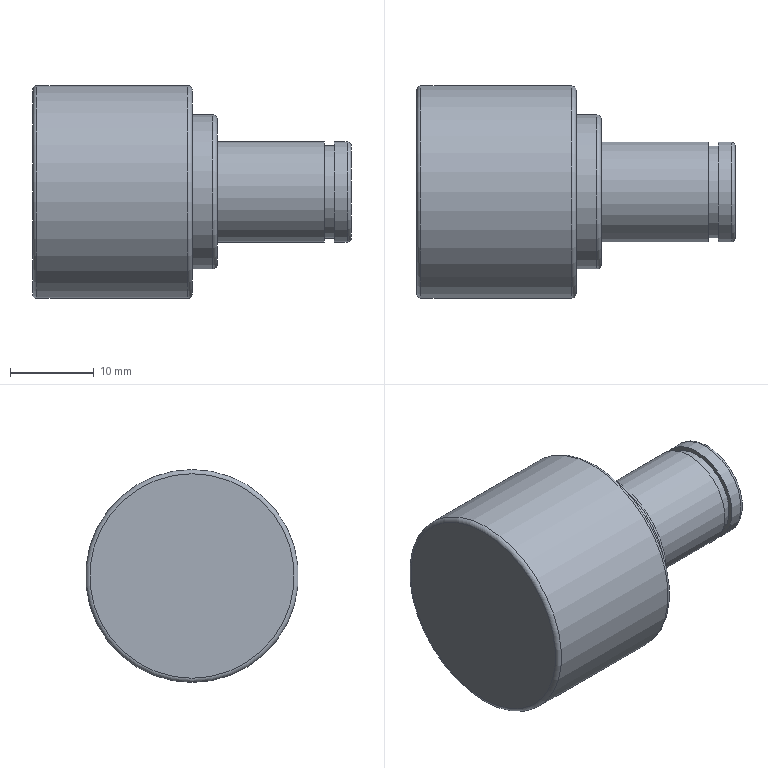Part | STEP file | 6100506 | 1 solid | 15 faces | box 38 x 25.4 x 25.4 mm | volume 12200 mm3 | plane 6 | cylinder 5 | torus 4 | commonest cylinder face diameters 12 x2 11 x1 18.4 x1 25.4 x1
STEP:
#1=CARTESIAN_POINT('',(0.,0.,0.));
#2=DIRECTION('',(0.,0.,1.));
#3=DIRECTION('',(1.,0.,0.));
#4=AXIS2_PLACEMENT_3D('',#1,#2,#3);
#5=CARTESIAN_POINT('',(0.,0.,12.2));
#6=VERTEX_POINT('',#5);
#7=CARTESIAN_POINT('',(0.,0.,0.));
#8=DIRECTION('',(-1.,0.,0.));
#9=DIRECTION('',(0.,0.,1.));
#10=AXIS2_PLACEMENT_3D('',#7,#8,#9);
#11=CIRCLE('',#10,12.2);
#12=CARTESIAN_POINT('',(0.,0.,0.));
#13=DIRECTION('',(1.,0.,0.));
#14=DIRECTION('',(0.,0.,-1.));
#15=AXIS2_PLACEMENT_3D('',#12,#13,#14);
#16=PLANE('',#15);
#17=CARTESIAN_POINT('',(-12.2,0.));
#18=CARTESIAN_POINT('',(-12.2,21.131));
#19=CARTESIAN_POINT('',(6.1,10.566));
#20=CARTESIAN_POINT('',(24.4,0.));
#21=CARTESIAN_POINT('',(6.1,-10.566));
#22=CARTESIAN_POINT('',(-12.2,-21.131));
#23=CARTESIAN_POINT('',(-12.2,0.));
#24=(BOUNDED_CURVE()B_SPLINE_CURVE(2,(#17,#18,#19,#20,#21,#22,#23),.UNSPECIFIED.,.T.,.F.)B_SPLINE_CURVE_WITH_KNOTS((1,2,2,2,2,1),(-2.094,0.,2.094,4.189,6.283,8.378),.UNSPECIFIED.)CURVE()GEOMETRIC_REPRESENTATION_ITEM()RATIONAL_B_SPLINE_CURVE((1.,0.5,1.,0.5,1.,0.5,1.))REPRESENTATION_ITEM(''));
#25=(GEOMETRIC_REPRESENTATION_CONTEXT(2)PARAMETRIC_REPRESENTATION_CONTEXT()REPRESENTATION_CONTEXT('',''));
#26=DEFINITIONAL_REPRESENTATION('',(#24),#25);
#27=PCURVE('',#16,#26);
#28=CARTESIAN_POINT('',(0.5,0.,0.));
#29=DIRECTION('',(-1.,0.,0.));
#30=DIRECTION('',(0.,0.,1.));
#31=AXIS2_PLACEMENT_3D('',#28,#29,#30);
#32=TOROIDAL_SURFACE('',#31,12.2,0.5);
#33=CARTESIAN_POINT('',(0.,7.854));
#34=DIRECTION('',(1.,0.));
#35=VECTOR('',#34,1.);
#36=LINE('',#33,#35);
#37=(GEOMETRIC_REPRESENTATION_CONTEXT(2)PARAMETRIC_REPRESENTATION_CONTEXT()REPRESENTATION_CONTEXT('',''));
#38=DEFINITIONAL_REPRESENTATION('',(#36),#37);
#39=PCURVE('',#32,#38);
#40=SURFACE_CURVE('',#11,(#27,#39),.PCURVE_S1.);
#41=EDGE_CURVE('',#6,#6,#40,.T.);
#42=ORIENTED_EDGE('',*,*,#41,.T.);
#43=EDGE_LOOP('',(#42));
#44=FACE_BOUND('',#43,.T.);
#45=ADVANCED_FACE('',(#44),#16,.F.);
#46=ORIENTED_EDGE('',*,*,#41,.F.);
#47=CARTESIAN_POINT('',(0.5,0.,12.7));
#48=VERTEX_POINT('',#47);
#49=CARTESIAN_POINT('',(0.5,0.,12.7));
#50=CARTESIAN_POINT('',(0.3663,0.,12.7));
#51=CARTESIAN_POINT('',(0.2361,0.,12.657));
#52=CARTESIAN_POINT('',(0.124,0.,12.576));
#53=CARTESIAN_POINT('',(0.0425,0.,12.464));
#54=CARTESIAN_POINT('',(0.,0.,12.334));
#55=CARTESIAN_POINT('',(0.,0.,12.2));
#56=(BOUNDED_CURVE()B_SPLINE_CURVE(6,(#49,#50,#51,#52,#53,#54,#55),.UNSPECIFIED.,.F.,.F.)B_SPLINE_CURVE_WITH_KNOTS((7,7),(0.,1.571),.PIECEWISE_BEZIER_KNOTS.)CURVE()GEOMETRIC_REPRESENTATION_ITEM()RATIONAL_B_SPLINE_CURVE((1.031,1.01,0.9979,0.994,0.9979,1.01,1.031))REPRESENTATION_ITEM(''));
#57=CARTESIAN_POINT('',(0.,6.283));
#58=DIRECTION('',(0.,1.));
#59=VECTOR('',#58,1.);
#60=LINE('',#57,#59);
#61=(GEOMETRIC_REPRESENTATION_CONTEXT(2)PARAMETRIC_REPRESENTATION_CONTEXT()REPRESENTATION_CONTEXT('',''));
#62=DEFINITIONAL_REPRESENTATION('',(#60),#61);
#63=PCURVE('',#32,#62);
#64=CARTESIAN_POINT('',(6.283,6.283));
#65=DIRECTION('',(0.,1.));
#66=VECTOR('',#65,1.);
#67=LINE('',#64,#66);
#68=(GEOMETRIC_REPRESENTATION_CONTEXT(2)PARAMETRIC_REPRESENTATION_CONTEXT()REPRESENTATION_CONTEXT('',''));
#69=DEFINITIONAL_REPRESENTATION('',(#67),#68);
#70=PCURVE('',#32,#69);
#71=SEAM_CURVE('',#56,(#63,#70),.PCURVE_S1.);
#72=EDGE_CURVE('',#48,#6,#71,.T.);
#73=ORIENTED_EDGE('',*,*,#72,.F.);
#74=CARTESIAN_POINT('',(0.5,0.,0.));
#75=DIRECTION('',(-1.,0.,0.));
#76=DIRECTION('',(0.,0.,1.));
#77=AXIS2_PLACEMENT_3D('',#74,#75,#76);
#78=CIRCLE('',#77,12.7);
#79=CARTESIAN_POINT('',(0.,6.283));
#80=DIRECTION('',(1.,0.));
#81=VECTOR('',#80,1.);
#82=LINE('',#79,#81);
#83=(GEOMETRIC_REPRESENTATION_CONTEXT(2)PARAMETRIC_REPRESENTATION_CONTEXT()REPRESENTATION_CONTEXT('',''));
#84=DEFINITIONAL_REPRESENTATION('',(#82),#83);
#85=PCURVE('',#32,#84);
#86=CARTESIAN_POINT('',(0.,0.,0.));
#87=DIRECTION('',(-1.,0.,0.));
#88=DIRECTION('',(0.,0.,1.));
#89=AXIS2_PLACEMENT_3D('',#86,#87,#88);
#90=CYLINDRICAL_SURFACE('',#89,12.7);
#91=CARTESIAN_POINT('',(0.,-0.5));
#92=DIRECTION('',(1.,0.));
#93=VECTOR('',#92,1.);
#94=LINE('',#91,#93);
#95=(GEOMETRIC_REPRESENTATION_CONTEXT(2)PARAMETRIC_REPRESENTATION_CONTEXT()REPRESENTATION_CONTEXT('',''));
#96=DEFINITIONAL_REPRESENTATION('',(#94),#95);
#97=PCURVE('',#90,#96);
#98=SURFACE_CURVE('',#78,(#85,#97),.PCURVE_S1.);
#99=EDGE_CURVE('',#48,#48,#98,.T.);
#100=ORIENTED_EDGE('',*,*,#99,.T.);
#101=ORIENTED_EDGE('',*,*,#72,.T.);
#102=EDGE_LOOP('',(#46,#73,#100,#101));
#103=FACE_BOUND('',#102,.T.);
#104=ADVANCED_FACE('',(#103),#32,.T.);
#105=ORIENTED_EDGE('',*,*,#99,.F.);
#106=CARTESIAN_POINT('',(18.5,0.,12.7));
#107=VERTEX_POINT('',#106);
#108=CARTESIAN_POINT('',(18.5,0.,12.7));
#109=CARTESIAN_POINT('',(0.5,0.,12.7));
#110=B_SPLINE_CURVE_WITH_KNOTS('',1,(#108,#109),.UNSPECIFIED.,.F.,.F.,(2,2),(-18.5,-0.5),.PIECEWISE_BEZIER_KNOTS.);
#111=CARTESIAN_POINT('',(0.,0.));
#112=DIRECTION('',(0.,1.));
#113=VECTOR('',#112,1.);
#114=LINE('',#111,#113);
#115=(GEOMETRIC_REPRESENTATION_CONTEXT(2)PARAMETRIC_REPRESENTATION_CONTEXT()REPRESENTATION_CONTEXT('',''));
#116=DEFINITIONAL_REPRESENTATION('',(#114),#115);
#117=PCURVE('',#90,#116);
#118=CARTESIAN_POINT('',(6.283,0.));
#119=DIRECTION('',(0.,1.));
#120=VECTOR('',#119,1.);
#121=LINE('',#118,#120);
#122=(GEOMETRIC_REPRESENTATION_CONTEXT(2)PARAMETRIC_REPRESENTATION_CONTEXT()REPRESENTATION_CONTEXT('',''));
#123=DEFINITIONAL_REPRESENTATION('',(#121),#122);
#124=PCURVE('',#90,#123);
#125=SEAM_CURVE('',#110,(#117,#124),.PCURVE_S1.);
#126=EDGE_CURVE('',#107,#48,#125,.T.);
#127=ORIENTED_EDGE('',*,*,#126,.F.);
#128=CARTESIAN_POINT('',(18.5,0.,0.));
#129=DIRECTION('',(-1.,0.,0.));
#130=DIRECTION('',(0.,0.,1.));
#131=AXIS2_PLACEMENT_3D('',#128,#129,#130);
#132=CIRCLE('',#131,12.7);
#133=CARTESIAN_POINT('',(0.,-18.5));
#134=DIRECTION('',(1.,0.));
#135=VECTOR('',#134,1.);
#136=LINE('',#133,#135);
#137=(GEOMETRIC_REPRESENTATION_CONTEXT(2)PARAMETRIC_REPRESENTATION_CONTEXT()REPRESENTATION_CONTEXT('',''));
#138=DEFINITIONAL_REPRESENTATION('',(#136),#137);
#139=PCURVE('',#90,#138);
#140=CARTESIAN_POINT('',(18.5,0.,0.));
#141=DIRECTION('',(-1.,0.,0.));
#142=DIRECTION('',(0.,0.,1.));
#143=AXIS2_PLACEMENT_3D('',#140,#141,#142);
#144=TOROIDAL_SURFACE('',#143,12.2,0.5);
#145=CARTESIAN_POINT('',(0.,6.283));
#146=DIRECTION('',(1.,0.));
#147=VECTOR('',#146,1.);
#148=LINE('',#145,#147);
#149=(GEOMETRIC_REPRESENTATION_CONTEXT(2)PARAMETRIC_REPRESENTATION_CONTEXT()REPRESENTATION_CONTEXT('',''));
#150=DEFINITIONAL_REPRESENTATION('',(#148),#149);
#151=PCURVE('',#144,#150);
#152=SURFACE_CURVE('',#132,(#139,#151),.PCURVE_S1.);
#153=EDGE_CURVE('',#107,#107,#152,.T.);
#154=ORIENTED_EDGE('',*,*,#153,.T.);
#155=ORIENTED_EDGE('',*,*,#126,.T.);
#156=EDGE_LOOP('',(#105,#127,#154,#155));
#157=FACE_BOUND('',#156,.T.);
#158=ADVANCED_FACE('',(#157),#90,.T.);
#159=ORIENTED_EDGE('',*,*,#153,.F.);
#160=CARTESIAN_POINT('',(19.,0.,12.2));
#161=VERTEX_POINT('',#160);
#162=CARTESIAN_POINT('',(19.,0.,12.2));
#163=CARTESIAN_POINT('',(19.,0.,12.334));
#164=CARTESIAN_POINT('',(18.957,0.,12.464));
#165=CARTESIAN_POINT('',(18.876,0.,12.576));
#166=CARTESIAN_POINT('',(18.764,0.,12.657));
#167=CARTESIAN_POINT('',(18.634,0.,12.7));
#168=CARTESIAN_POINT('',(18.5,0.,12.7));
#169=(BOUNDED_CURVE()B_SPLINE_CURVE(6,(#162,#163,#164,#165,#166,#167,#168),.UNSPECIFIED.,.F.,.F.)B_SPLINE_CURVE_WITH_KNOTS((7,7),(-1.571,0.),.PIECEWISE_BEZIER_KNOTS.)CURVE()GEOMETRIC_REPRESENTATION_ITEM()RATIONAL_B_SPLINE_CURVE((1.031,1.01,0.9979,0.994,0.9979,1.01,1.031))REPRESENTATION_ITEM(''));
#170=CARTESIAN_POINT('',(0.,6.283));
#171=DIRECTION('',(0.,1.));
#172=VECTOR('',#171,1.);
#173=LINE('',#170,#172);
#174=(GEOMETRIC_REPRESENTATION_CONTEXT(2)PARAMETRIC_REPRESENTATION_CONTEXT()REPRESENTATION_CONTEXT('',''));
#175=DEFINITIONAL_REPRESENTATION('',(#173),#174);
#176=PCURVE('',#144,#175);
#177=CARTESIAN_POINT('',(6.283,6.283));
#178=DIRECTION('',(0.,1.));
#179=VECTOR('',#178,1.);
#180=LINE('',#177,#179);
#181=(GEOMETRIC_REPRESENTATION_CONTEXT(2)PARAMETRIC_REPRESENTATION_CONTEXT()REPRESENTATION_CONTEXT('',''));
#182=DEFINITIONAL_REPRESENTATION('',(#180),#181);
#183=PCURVE('',#144,#182);
#184=SEAM_CURVE('',#169,(#176,#183),.PCURVE_S1.);
#185=EDGE_CURVE('',#161,#107,#184,.T.);
#186=ORIENTED_EDGE('',*,*,#185,.F.);
#187=CARTESIAN_POINT('',(19.,0.,0.));
#188=DIRECTION('',(-1.,0.,0.));
#189=DIRECTION('',(0.,0.,1.));
#190=AXIS2_PLACEMENT_3D('',#187,#188,#189);
#191=CIRCLE('',#190,12.2);
#192=CARTESIAN_POINT('',(0.,4.712));
#193=DIRECTION('',(1.,0.));
#194=VECTOR('',#193,1.);
#195=LINE('',#192,#194);
#196=(GEOMETRIC_REPRESENTATION_CONTEXT(2)PARAMETRIC_REPRESENTATION_CONTEXT()REPRESENTATION_CONTEXT('',''));
#197=DEFINITIONAL_REPRESENTATION('',(#195),#196);
#198=PCURVE('',#144,#197);
#199=CARTESIAN_POINT('',(19.,12.2,0.));
#200=DIRECTION('',(-1.,0.,0.));
#201=DIRECTION('',(0.,0.,1.));
#202=AXIS2_PLACEMENT_3D('',#199,#200,#201);
#203=PLANE('',#202);
#204=CARTESIAN_POINT('',(0.,-12.2));
#205=DIRECTION('',(1.,0.));
#206=AXIS2_PLACEMENT_2D('',#204,#205);
#207=CIRCLE('',#206,12.2);
#208=(GEOMETRIC_REPRESENTATION_CONTEXT(2)PARAMETRIC_REPRESENTATION_CONTEXT()REPRESENTATION_CONTEXT('',''));
#209=DEFINITIONAL_REPRESENTATION('',(#207),#208);
#210=PCURVE('',#203,#209);
#211=SURFACE_CURVE('',#191,(#198,#210),.PCURVE_S1.);
#212=EDGE_CURVE('',#161,#161,#211,.T.);
#213=ORIENTED_EDGE('',*,*,#212,.T.);
#214=ORIENTED_EDGE('',*,*,#185,.T.);
#215=EDGE_LOOP('',(#159,#186,#213,#214));
#216=FACE_BOUND('',#215,.T.);
#217=ADVANCED_FACE('',(#216),#144,.T.);
#218=ORIENTED_EDGE('',*,*,#212,.F.);
#219=EDGE_LOOP('',(#218));
#220=FACE_BOUND('',#219,.T.);
#221=CARTESIAN_POINT('',(19.,0.,9.2));
#222=VERTEX_POINT('',#221);
#223=CARTESIAN_POINT('',(19.,0.,0.));
#224=DIRECTION('',(-1.,0.,0.));
#225=DIRECTION('',(0.,0.,1.));
#226=AXIS2_PLACEMENT_3D('',#223,#224,#225);
#227=CIRCLE('',#226,9.2);
#228=CARTESIAN_POINT('',(0.,-12.2));
#229=DIRECTION('',(1.,0.));
#230=AXIS2_PLACEMENT_2D('',#228,#229);
#231=CIRCLE('',#230,9.2);
#232=(GEOMETRIC_REPRESENTATION_CONTEXT(2)PARAMETRIC_REPRESENTATION_CONTEXT()REPRESENTATION_CONTEXT('',''));
#233=DEFINITIONAL_REPRESENTATION('',(#231),#232);
#234=PCURVE('',#203,#233);
#235=CARTESIAN_POINT('',(0.,0.,0.));
#236=DIRECTION('',(-1.,0.,0.));
#237=DIRECTION('',(0.,0.,1.));
#238=AXIS2_PLACEMENT_3D('',#235,#236,#237);
#239=CYLINDRICAL_SURFACE('',#238,9.2);
#240=CARTESIAN_POINT('',(0.,-19.));
#241=DIRECTION('',(1.,0.));
#242=VECTOR('',#241,1.);
#243=LINE('',#240,#242);
#244=(GEOMETRIC_REPRESENTATION_CONTEXT(2)PARAMETRIC_REPRESENTATION_CONTEXT()REPRESENTATION_CONTEXT('',''));
#245=DEFINITIONAL_REPRESENTATION('',(#243),#244);
#246=PCURVE('',#239,#245);
#247=SURFACE_CURVE('',#227,(#234,#246),.PCURVE_S1.);
#248=EDGE_CURVE('',#222,#222,#247,.T.);
#249=ORIENTED_EDGE('',*,*,#248,.T.);
#250=EDGE_LOOP('',(#249));
#251=FACE_BOUND('',#250,.T.);
#252=ADVANCED_FACE('',(#220,#251),#203,.F.);
#253=ORIENTED_EDGE('',*,*,#248,.F.);
#254=CARTESIAN_POINT('',(21.5,0.,9.2));
#255=VERTEX_POINT('',#254);
#256=CARTESIAN_POINT('',(21.5,0.,9.2));
#257=CARTESIAN_POINT('',(19.,0.,9.2));
#258=B_SPLINE_CURVE_WITH_KNOTS('',1,(#256,#257),.UNSPECIFIED.,.F.,.F.,(2,2),(-21.5,-19.),.PIECEWISE_BEZIER_KNOTS.);
#259=CARTESIAN_POINT('',(0.,0.));
#260=DIRECTION('',(0.,1.));
#261=VECTOR('',#260,1.);
#262=LINE('',#259,#261);
#263=(GEOMETRIC_REPRESENTATION_CONTEXT(2)PARAMETRIC_REPRESENTATION_CONTEXT()REPRESENTATION_CONTEXT('',''));
#264=DEFINITIONAL_REPRESENTATION('',(#262),#263);
#265=PCURVE('',#239,#264);
#266=CARTESIAN_POINT('',(6.283,0.));
#267=DIRECTION('',(0.,1.));
#268=VECTOR('',#267,1.);
#269=LINE('',#266,#268);
#270=(GEOMETRIC_REPRESENTATION_CONTEXT(2)PARAMETRIC_REPRESENTATION_CONTEXT()REPRESENTATION_CONTEXT('',''));
#271=DEFINITIONAL_REPRESENTATION('',(#269),#270);
#272=PCURVE('',#239,#271);
#273=SEAM_CURVE('',#258,(#265,#272),.PCURVE_S1.);
#274=EDGE_CURVE('',#255,#222,#273,.T.);
#275=ORIENTED_EDGE('',*,*,#274,.F.);
#276=CARTESIAN_POINT('',(21.5,0.,0.));
#277=DIRECTION('',(-1.,0.,0.));
#278=DIRECTION('',(0.,0.,1.));
#279=AXIS2_PLACEMENT_3D('',#276,#277,#278);
#280=CIRCLE('',#279,9.2);
#281=CARTESIAN_POINT('',(0.,-21.5));
#282=DIRECTION('',(1.,0.));
#283=VECTOR('',#282,1.);
#284=LINE('',#281,#283);
#285=(GEOMETRIC_REPRESENTATION_CONTEXT(2)PARAMETRIC_REPRESENTATION_CONTEXT()REPRESENTATION_CONTEXT('',''));
#286=DEFINITIONAL_REPRESENTATION('',(#284),#285);
#287=PCURVE('',#239,#286);
#288=CARTESIAN_POINT('',(21.5,0.,0.));
#289=DIRECTION('',(-1.,0.,0.));
#290=DIRECTION('',(0.,0.,1.));
#291=AXIS2_PLACEMENT_3D('',#288,#289,#290);
#292=TOROIDAL_SURFACE('',#291,8.7,0.5);
#293=CARTESIAN_POINT('',(0.,6.283));
#294=DIRECTION('',(1.,0.));
#295=VECTOR('',#294,1.);
#296=LINE('',#293,#295);
#297=(GEOMETRIC_REPRESENTATION_CONTEXT(2)PARAMETRIC_REPRESENTATION_CONTEXT()REPRESENTATION_CONTEXT('',''));
#298=DEFINITIONAL_REPRESENTATION('',(#296),#297);
#299=PCURVE('',#292,#298);
#300=SURFACE_CURVE('',#280,(#287,#299),.PCURVE_S1.);
#301=EDGE_CURVE('',#255,#255,#300,.T.);
#302=ORIENTED_EDGE('',*,*,#301,.T.);
#303=ORIENTED_EDGE('',*,*,#274,.T.);
#304=EDGE_LOOP('',(#253,#275,#302,#303));
#305=FACE_BOUND('',#304,.T.);
#306=ADVANCED_FACE('',(#305),#239,.T.);
#307=ORIENTED_EDGE('',*,*,#301,.F.);
#308=CARTESIAN_POINT('',(22.,0.,8.7));
#309=VERTEX_POINT('',#308);
#310=CARTESIAN_POINT('',(22.,0.,8.7));
#311=CARTESIAN_POINT('',(22.,0.,8.834));
#312=CARTESIAN_POINT('',(21.957,0.,8.964));
#313=CARTESIAN_POINT('',(21.876,0.,9.076));
#314=CARTESIAN_POINT('',(21.764,0.,9.157));
#315=CARTESIAN_POINT('',(21.634,0.,9.2));
#316=CARTESIAN_POINT('',(21.5,0.,9.2));
#317=(BOUNDED_CURVE()B_SPLINE_CURVE(6,(#310,#311,#312,#313,#314,#315,#316),.UNSPECIFIED.,.F.,.F.)B_SPLINE_CURVE_WITH_KNOTS((7,7),(-1.571,0.),.PIECEWISE_BEZIER_KNOTS.)CURVE()GEOMETRIC_REPRESENTATION_ITEM()RATIONAL_B_SPLINE_CURVE((1.031,1.01,0.9979,0.994,0.9979,1.01,1.031))REPRESENTATION_ITEM(''));
#318=CARTESIAN_POINT('',(0.,6.283));
#319=DIRECTION('',(0.,1.));
#320=VECTOR('',#319,1.);
#321=LINE('',#318,#320);
#322=(GEOMETRIC_REPRESENTATION_CONTEXT(2)PARAMETRIC_REPRESENTATION_CONTEXT()REPRESENTATION_CONTEXT('',''));
#323=DEFINITIONAL_REPRESENTATION('',(#321),#322);
#324=PCURVE('',#292,#323);
#325=CARTESIAN_POINT('',(6.283,6.283));
#326=DIRECTION('',(0.,1.));
#327=VECTOR('',#326,1.);
#328=LINE('',#325,#327);
#329=(GEOMETRIC_REPRESENTATION_CONTEXT(2)PARAMETRIC_REPRESENTATION_CONTEXT()REPRESENTATION_CONTEXT('',''));
#330=DEFINITIONAL_REPRESENTATION('',(#328),#329);
#331=PCURVE('',#292,#330);
#332=SEAM_CURVE('',#317,(#324,#331),.PCURVE_S1.);
#333=EDGE_CURVE('',#309,#255,#332,.T.);
#334=ORIENTED_EDGE('',*,*,#333,.F.);
#335=CARTESIAN_POINT('',(22.,0.,0.));
#336=DIRECTION('',(-1.,0.,0.));
#337=DIRECTION('',(0.,0.,1.));
#338=AXIS2_PLACEMENT_3D('',#335,#336,#337);
#339=CIRCLE('',#338,8.7);
#340=CARTESIAN_POINT('',(0.,4.712));
#341=DIRECTION('',(1.,0.));
#342=VECTOR('',#341,1.);
#343=LINE('',#340,#342);
#344=(GEOMETRIC_REPRESENTATION_CONTEXT(2)PARAMETRIC_REPRESENTATION_CONTEXT()REPRESENTATION_CONTEXT('',''));
#345=DEFINITIONAL_REPRESENTATION('',(#343),#344);
#346=PCURVE('',#292,#345);
#347=CARTESIAN_POINT('',(22.,8.7,0.));
#348=DIRECTION('',(-1.,0.,0.));
#349=DIRECTION('',(0.,0.,1.));
#350=AXIS2_PLACEMENT_3D('',#347,#348,#349);
#351=PLANE('',#350);
#352=CARTESIAN_POINT('',(0.,-8.7));
#353=DIRECTION('',(1.,0.));
#354=AXIS2_PLACEMENT_2D('',#352,#353);
#355=CIRCLE('',#354,8.7);
#356=(GEOMETRIC_REPRESENTATION_CONTEXT(2)PARAMETRIC_REPRESENTATION_CONTEXT()REPRESENTATION_CONTEXT('',''));
#357=DEFINITIONAL_REPRESENTATION('',(#355),#356);
#358=PCURVE('',#351,#357);
#359=SURFACE_CURVE('',#339,(#346,#358),.PCURVE_S1.);
#360=EDGE_CURVE('',#309,#309,#359,.T.);
#361=ORIENTED_EDGE('',*,*,#360,.T.);
#362=ORIENTED_EDGE('',*,*,#333,.T.);
#363=EDGE_LOOP('',(#307,#334,#361,#362));
#364=FACE_BOUND('',#363,.T.);
#365=ADVANCED_FACE('',(#364),#292,.T.);
#366=ORIENTED_EDGE('',*,*,#360,.F.);
#367=EDGE_LOOP('',(#366));
#368=FACE_BOUND('',#367,.T.);
#369=CARTESIAN_POINT('',(22.,0.,6.));
#370=VERTEX_POINT('',#369);
#371=CARTESIAN_POINT('',(22.,0.,0.));
#372=DIRECTION('',(-1.,0.,0.));
#373=DIRECTION('',(0.,0.,1.));
#374=AXIS2_PLACEMENT_3D('',#371,#372,#373);
#375=CIRCLE('',#374,6.);
#376=CARTESIAN_POINT('',(0.,-8.7));
#377=DIRECTION('',(1.,0.));
#378=AXIS2_PLACEMENT_2D('',#376,#377);
#379=CIRCLE('',#378,6.);
#380=(GEOMETRIC_REPRESENTATION_CONTEXT(2)PARAMETRIC_REPRESENTATION_CONTEXT()REPRESENTATION_CONTEXT('',''));
#381=DEFINITIONAL_REPRESENTATION('',(#379),#380);
#382=PCURVE('',#351,#381);
#383=CARTESIAN_POINT('',(0.,0.,0.));
#384=DIRECTION('',(-1.,0.,0.));
#385=DIRECTION('',(0.,0.,1.));
#386=AXIS2_PLACEMENT_3D('',#383,#384,#385);
#387=CYLINDRICAL_SURFACE('',#386,6.);
#388=CARTESIAN_POINT('',(0.,-22.));
#389=DIRECTION('',(1.,0.));
#390=VECTOR('',#389,1.);
#391=LINE('',#388,#390);
#392=(GEOMETRIC_REPRESENTATION_CONTEXT(2)PARAMETRIC_REPRESENTATION_CONTEXT()REPRESENTATION_CONTEXT('',''));
#393=DEFINITIONAL_REPRESENTATION('',(#391),#392);
#394=PCURVE('',#387,#393);
#395=SURFACE_CURVE('',#375,(#382,#394),.PCURVE_S1.);
#396=EDGE_CURVE('',#370,#370,#395,.T.);
#397=ORIENTED_EDGE('',*,*,#396,.T.);
#398=EDGE_LOOP('',(#397));
#399=FACE_BOUND('',#398,.T.);
#400=ADVANCED_FACE('',(#368,#399),#351,.F.);
#401=ORIENTED_EDGE('',*,*,#396,.F.);
#402=CARTESIAN_POINT('',(34.8,0.,6.));
#403=VERTEX_POINT('',#402);
#404=CARTESIAN_POINT('',(34.8,0.,6.));
#405=CARTESIAN_POINT('',(22.,0.,6.));
#406=B_SPLINE_CURVE_WITH_KNOTS('',1,(#404,#405),.UNSPECIFIED.,.F.,.F.,(2,2),(-34.8,-22.),.PIECEWISE_BEZIER_KNOTS.);
#407=CARTESIAN_POINT('',(0.,0.));
#408=DIRECTION('',(0.,1.));
#409=VECTOR('',#408,1.);
#410=LINE('',#407,#409);
#411=(GEOMETRIC_REPRESENTATION_CONTEXT(2)PARAMETRIC_REPRESENTATION_CONTEXT()REPRESENTATION_CONTEXT('',''));
#412=DEFINITIONAL_REPRESENTATION('',(#410),#411);
#413=PCURVE('',#387,#412);
#414=CARTESIAN_POINT('',(6.283,0.));
#415=DIRECTION('',(0.,1.));
#416=VECTOR('',#415,1.);
#417=LINE('',#414,#416);
#418=(GEOMETRIC_REPRESENTATION_CONTEXT(2)PARAMETRIC_REPRESENTATION_CONTEXT()REPRESENTATION_CONTEXT('',''));
#419=DEFINITIONAL_REPRESENTATION('',(#417),#418);
#420=PCURVE('',#387,#419);
#421=SEAM_CURVE('',#406,(#413,#420),.PCURVE_S1.);
#422=EDGE_CURVE('',#403,#370,#421,.T.);
#423=ORIENTED_EDGE('',*,*,#422,.F.);
#424=CARTESIAN_POINT('',(34.8,0.,0.));
#425=DIRECTION('',(-1.,0.,0.));
#426=DIRECTION('',(0.,0.,1.));
#427=AXIS2_PLACEMENT_3D('',#424,#425,#426);
#428=CIRCLE('',#427,6.);
#429=CARTESIAN_POINT('',(0.,-34.8));
#430=DIRECTION('',(1.,0.));
#431=VECTOR('',#430,1.);
#432=LINE('',#429,#431);
#433=(GEOMETRIC_REPRESENTATION_CONTEXT(2)PARAMETRIC_REPRESENTATION_CONTEXT()REPRESENTATION_CONTEXT('',''));
#434=DEFINITIONAL_REPRESENTATION('',(#432),#433);
#435=PCURVE('',#387,#434);
#436=CARTESIAN_POINT('',(34.8,6.,0.));
#437=DIRECTION('',(-1.,0.,0.));
#438=DIRECTION('',(0.,0.,1.));
#439=AXIS2_PLACEMENT_3D('',#436,#437,#438);
#440=PLANE('',#439);
#441=CARTESIAN_POINT('',(0.,-6.));
#442=DIRECTION('',(1.,0.));
#443=AXIS2_PLACEMENT_2D('',#441,#442);
#444=CIRCLE('',#443,6.);
#445=(GEOMETRIC_REPRESENTATION_CONTEXT(2)PARAMETRIC_REPRESENTATION_CONTEXT()REPRESENTATION_CONTEXT('',''));
#446=DEFINITIONAL_REPRESENTATION('',(#444),#445);
#447=PCURVE('',#440,#446);
#448=SURFACE_CURVE('',#428,(#435,#447),.PCURVE_S1.);
#449=EDGE_CURVE('',#403,#403,#448,.T.);
#450=ORIENTED_EDGE('',*,*,#449,.T.);
#451=ORIENTED_EDGE('',*,*,#422,.T.);
#452=EDGE_LOOP('',(#401,#423,#450,#451));
#453=FACE_BOUND('',#452,.T.);
#454=ADVANCED_FACE('',(#453),#387,.T.);
#455=ORIENTED_EDGE('',*,*,#449,.F.);
#456=EDGE_LOOP('',(#455));
#457=FACE_BOUND('',#456,.T.);
#458=CARTESIAN_POINT('',(34.8,0.,5.5));
#459=VERTEX_POINT('',#458);
#460=CARTESIAN_POINT('',(34.8,0.,0.));
#461=DIRECTION('',(-1.,0.,0.));
#462=DIRECTION('',(0.,0.,1.));
#463=AXIS2_PLACEMENT_3D('',#460,#461,#462);
#464=CIRCLE('',#463,5.5);
#465=CARTESIAN_POINT('',(0.,-6.));
#466=DIRECTION('',(1.,0.));
#467=AXIS2_PLACEMENT_2D('',#465,#466);
#468=CIRCLE('',#467,5.5);
#469=(GEOMETRIC_REPRESENTATION_CONTEXT(2)PARAMETRIC_REPRESENTATION_CONTEXT()REPRESENTATION_CONTEXT('',''));
#470=DEFINITIONAL_REPRESENTATION('',(#468),#469);
#471=PCURVE('',#440,#470);
#472=CARTESIAN_POINT('',(0.,0.,0.));
#473=DIRECTION('',(-1.,0.,0.));
#474=DIRECTION('',(0.,0.,1.));
#475=AXIS2_PLACEMENT_3D('',#472,#473,#474);
#476=CYLINDRICAL_SURFACE('',#475,5.5);
#477=CARTESIAN_POINT('',(0.,-34.8));
#478=DIRECTION('',(1.,0.));
#479=VECTOR('',#478,1.);
#480=LINE('',#477,#479);
#481=(GEOMETRIC_REPRESENTATION_CONTEXT(2)PARAMETRIC_REPRESENTATION_CONTEXT()REPRESENTATION_CONTEXT('',''));
#482=DEFINITIONAL_REPRESENTATION('',(#480),#481);
#483=PCURVE('',#476,#482);
#484=SURFACE_CURVE('',#464,(#471,#483),.PCURVE_S1.);
#485=EDGE_CURVE('',#459,#459,#484,.T.);
#486=ORIENTED_EDGE('',*,*,#485,.T.);
#487=EDGE_LOOP('',(#486));
#488=FACE_BOUND('',#487,.T.);
#489=ADVANCED_FACE('',(#457,#488),#440,.F.);
#490=ORIENTED_EDGE('',*,*,#485,.F.);
#491=CARTESIAN_POINT('',(36.,0.,5.5));
#492=VERTEX_POINT('',#491);
#493=CARTESIAN_POINT('',(36.,0.,5.5));
#494=CARTESIAN_POINT('',(34.8,0.,5.5));
#495=B_SPLINE_CURVE_WITH_KNOTS('',1,(#493,#494),.UNSPECIFIED.,.F.,.F.,(2,2),(-36.,-34.8),.PIECEWISE_BEZIER_KNOTS.);
#496=CARTESIAN_POINT('',(0.,0.));
#497=DIRECTION('',(0.,1.));
#498=VECTOR('',#497,1.);
#499=LINE('',#496,#498);
#500=(GEOMETRIC_REPRESENTATION_CONTEXT(2)PARAMETRIC_REPRESENTATION_CONTEXT()REPRESENTATION_CONTEXT('',''));
#501=DEFINITIONAL_REPRESENTATION('',(#499),#500);
#502=PCURVE('',#476,#501);
#503=CARTESIAN_POINT('',(6.283,0.));
#504=DIRECTION('',(0.,1.));
#505=VECTOR('',#504,1.);
#506=LINE('',#503,#505);
#507=(GEOMETRIC_REPRESENTATION_CONTEXT(2)PARAMETRIC_REPRESENTATION_CONTEXT()REPRESENTATION_CONTEXT('',''));
#508=DEFINITIONAL_REPRESENTATION('',(#506),#507);
#509=PCURVE('',#476,#508);
#510=SEAM_CURVE('',#495,(#502,#509),.PCURVE_S1.);
#511=EDGE_CURVE('',#492,#459,#510,.T.);
#512=ORIENTED_EDGE('',*,*,#511,.F.);
#513=CARTESIAN_POINT('',(36.,0.,0.));
#514=DIRECTION('',(-1.,0.,0.));
#515=DIRECTION('',(0.,0.,1.));
#516=AXIS2_PLACEMENT_3D('',#513,#514,#515);
#517=CIRCLE('',#516,5.5);
#518=CARTESIAN_POINT('',(0.,-36.));
#519=DIRECTION('',(1.,0.));
#520=VECTOR('',#519,1.);
#521=LINE('',#518,#520);
#522=(GEOMETRIC_REPRESENTATION_CONTEXT(2)PARAMETRIC_REPRESENTATION_CONTEXT()REPRESENTATION_CONTEXT('',''));
#523=DEFINITIONAL_REPRESENTATION('',(#521),#522);
#524=PCURVE('',#476,#523);
#525=CARTESIAN_POINT('',(36.,5.5,0.));
#526=DIRECTION('',(1.,0.,0.));
#527=DIRECTION('',(0.,0.,-1.));
#528=AXIS2_PLACEMENT_3D('',#525,#526,#527);
#529=PLANE('',#528);
#530=CARTESIAN_POINT('',(-5.5,-5.5));
#531=CARTESIAN_POINT('',(-5.5,4.026));
#532=CARTESIAN_POINT('',(2.75,-0.7369));
#533=CARTESIAN_POINT('',(11.,-5.5));
#534=CARTESIAN_POINT('',(2.75,-10.263));
#535=CARTESIAN_POINT('',(-5.5,-15.026));
#536=CARTESIAN_POINT('',(-5.5,-5.5));
#537=(BOUNDED_CURVE()B_SPLINE_CURVE(2,(#530,#531,#532,#533,#534,#535,#536),.UNSPECIFIED.,.T.,.F.)B_SPLINE_CURVE_WITH_KNOTS((1,2,2,2,2,1),(-2.094,0.,2.094,4.189,6.283,8.378),.UNSPECIFIED.)CURVE()GEOMETRIC_REPRESENTATION_ITEM()RATIONAL_B_SPLINE_CURVE((1.,0.5,1.,0.5,1.,0.5,1.))REPRESENTATION_ITEM(''));
#538=(GEOMETRIC_REPRESENTATION_CONTEXT(2)PARAMETRIC_REPRESENTATION_CONTEXT()REPRESENTATION_CONTEXT('',''));
#539=DEFINITIONAL_REPRESENTATION('',(#537),#538);
#540=PCURVE('',#529,#539);
#541=SURFACE_CURVE('',#517,(#524,#540),.PCURVE_S1.);
#542=EDGE_CURVE('',#492,#492,#541,.T.);
#543=ORIENTED_EDGE('',*,*,#542,.T.);
#544=ORIENTED_EDGE('',*,*,#511,.T.);
#545=EDGE_LOOP('',(#490,#512,#543,#544));
#546=FACE_BOUND('',#545,.T.);
#547=ADVANCED_FACE('',(#546),#476,.T.);
#548=ORIENTED_EDGE('',*,*,#542,.F.);
#549=EDGE_LOOP('',(#548));
#550=FACE_BOUND('',#549,.T.);
#551=CARTESIAN_POINT('',(36.,0.,6.));
#552=VERTEX_POINT('',#551);
#553=CARTESIAN_POINT('',(36.,0.,0.));
#554=DIRECTION('',(-1.,0.,0.));
#555=DIRECTION('',(0.,0.,1.));
#556=AXIS2_PLACEMENT_3D('',#553,#554,#555);
#557=CIRCLE('',#556,6.);
#558=CARTESIAN_POINT('',(-6.,-5.5));
#559=CARTESIAN_POINT('',(-6.,4.892));
#560=CARTESIAN_POINT('',(3.,-0.3038));
#561=CARTESIAN_POINT('',(12.,-5.5));
#562=CARTESIAN_POINT('',(3.,-10.696));
#563=CARTESIAN_POINT('',(-6.,-15.892));
#564=CARTESIAN_POINT('',(-6.,-5.5));
#565=(BOUNDED_CURVE()B_SPLINE_CURVE(2,(#558,#559,#560,#561,#562,#563,#564),.UNSPECIFIED.,.T.,.F.)B_SPLINE_CURVE_WITH_KNOTS((1,2,2,2,2,1),(-2.094,0.,2.094,4.189,6.283,8.378),.UNSPECIFIED.)CURVE()GEOMETRIC_REPRESENTATION_ITEM()RATIONAL_B_SPLINE_CURVE((1.,0.5,1.,0.5,1.,0.5,1.))REPRESENTATION_ITEM(''));
#566=(GEOMETRIC_REPRESENTATION_CONTEXT(2)PARAMETRIC_REPRESENTATION_CONTEXT()REPRESENTATION_CONTEXT('',''));
#567=DEFINITIONAL_REPRESENTATION('',(#565),#566);
#568=PCURVE('',#529,#567);
#569=CARTESIAN_POINT('',(0.,0.,0.));
#570=DIRECTION('',(-1.,0.,0.));
#571=DIRECTION('',(0.,0.,1.));
#572=AXIS2_PLACEMENT_3D('',#569,#570,#571);
#573=CYLINDRICAL_SURFACE('',#572,6.);
#574=CARTESIAN_POINT('',(0.,-36.));
#575=DIRECTION('',(1.,0.));
#576=VECTOR('',#575,1.);
#577=LINE('',#574,#576);
#578=(GEOMETRIC_REPRESENTATION_CONTEXT(2)PARAMETRIC_REPRESENTATION_CONTEXT()REPRESENTATION_CONTEXT('',''));
#579=DEFINITIONAL_REPRESENTATION('',(#577),#578);
#580=PCURVE('',#573,#579);
#581=SURFACE_CURVE('',#557,(#568,#580),.PCURVE_S1.);
#582=EDGE_CURVE('',#552,#552,#581,.T.);
#583=ORIENTED_EDGE('',*,*,#582,.T.);
#584=EDGE_LOOP('',(#583));
#585=FACE_BOUND('',#584,.T.);
#586=ADVANCED_FACE('',(#550,#585),#529,.F.);
#587=ORIENTED_EDGE('',*,*,#582,.F.);
#588=CARTESIAN_POINT('',(37.5,0.,6.));
#589=VERTEX_POINT('',#588);
#590=CARTESIAN_POINT('',(37.5,0.,6.));
#591=CARTESIAN_POINT('',(36.,0.,6.));
#592=B_SPLINE_CURVE_WITH_KNOTS('',1,(#590,#591),.UNSPECIFIED.,.F.,.F.,(2,2),(-37.5,-36.),.PIECEWISE_BEZIER_KNOTS.);
#593=CARTESIAN_POINT('',(0.,0.));
#594=DIRECTION('',(0.,1.));
#595=VECTOR('',#594,1.);
#596=LINE('',#593,#595);
#597=(GEOMETRIC_REPRESENTATION_CONTEXT(2)PARAMETRIC_REPRESENTATION_CONTEXT()REPRESENTATION_CONTEXT('',''));
#598=DEFINITIONAL_REPRESENTATION('',(#596),#597);
#599=PCURVE('',#573,#598);
#600=CARTESIAN_POINT('',(6.283,0.));
#601=DIRECTION('',(0.,1.));
#602=VECTOR('',#601,1.);
#603=LINE('',#600,#602);
#604=(GEOMETRIC_REPRESENTATION_CONTEXT(2)PARAMETRIC_REPRESENTATION_CONTEXT()REPRESENTATION_CONTEXT('',''));
#605=DEFINITIONAL_REPRESENTATION('',(#603),#604);
#606=PCURVE('',#573,#605);
#607=SEAM_CURVE('',#592,(#599,#606),.PCURVE_S1.);
#608=EDGE_CURVE('',#589,#552,#607,.T.);
#609=ORIENTED_EDGE('',*,*,#608,.F.);
#610=CARTESIAN_POINT('',(37.5,0.,0.));
#611=DIRECTION('',(-1.,0.,0.));
#612=DIRECTION('',(0.,0.,1.));
#613=AXIS2_PLACEMENT_3D('',#610,#611,#612);
#614=CIRCLE('',#613,6.);
#615=CARTESIAN_POINT('',(0.,-37.5));
#616=DIRECTION('',(1.,0.));
#617=VECTOR('',#616,1.);
#618=LINE('',#615,#617);
#619=(GEOMETRIC_REPRESENTATION_CONTEXT(2)PARAMETRIC_REPRESENTATION_CONTEXT()REPRESENTATION_CONTEXT('',''));
#620=DEFINITIONAL_REPRESENTATION('',(#618),#619);
#621=PCURVE('',#573,#620);
#622=CARTESIAN_POINT('',(37.5,0.,0.));
#623=DIRECTION('',(-1.,0.,0.));
#624=DIRECTION('',(0.,0.,1.));
#625=AXIS2_PLACEMENT_3D('',#622,#623,#624);
#626=TOROIDAL_SURFACE('',#625,5.5,0.5);
#627=CARTESIAN_POINT('',(0.,6.283));
#628=DIRECTION('',(1.,0.));
#629=VECTOR('',#628,1.);
#630=LINE('',#627,#629);
#631=(GEOMETRIC_REPRESENTATION_CONTEXT(2)PARAMETRIC_REPRESENTATION_CONTEXT()REPRESENTATION_CONTEXT('',''));
#632=DEFINITIONAL_REPRESENTATION('',(#630),#631);
#633=PCURVE('',#626,#632);
#634=SURFACE_CURVE('',#614,(#621,#633),.PCURVE_S1.);
#635=EDGE_CURVE('',#589,#589,#634,.T.);
#636=ORIENTED_EDGE('',*,*,#635,.T.);
#637=ORIENTED_EDGE('',*,*,#608,.T.);
#638=EDGE_LOOP('',(#587,#609,#636,#637));
#639=FACE_BOUND('',#638,.T.);
#640=ADVANCED_FACE('',(#639),#573,.T.);
#641=ORIENTED_EDGE('',*,*,#635,.F.);
#642=CARTESIAN_POINT('',(38.,0.,5.5));
#643=VERTEX_POINT('',#642);
#644=CARTESIAN_POINT('',(38.,0.,5.5));
#645=CARTESIAN_POINT('',(38.,0.,5.634));
#646=CARTESIAN_POINT('',(37.957,0.,5.764));
#647=CARTESIAN_POINT('',(37.876,0.,5.876));
#648=CARTESIAN_POINT('',(37.764,0.,5.957));
#649=CARTESIAN_POINT('',(37.634,0.,6.));
#650=CARTESIAN_POINT('',(37.5,0.,6.));
#651=(BOUNDED_CURVE()B_SPLINE_CURVE(6,(#644,#645,#646,#647,#648,#649,#650),.UNSPECIFIED.,.F.,.F.)B_SPLINE_CURVE_WITH_KNOTS((7,7),(-1.571,0.),.PIECEWISE_BEZIER_KNOTS.)CURVE()GEOMETRIC_REPRESENTATION_ITEM()RATIONAL_B_SPLINE_CURVE((1.031,1.01,0.9979,0.994,0.9979,1.01,1.031))REPRESENTATION_ITEM(''));
#652=CARTESIAN_POINT('',(0.,6.283));
#653=DIRECTION('',(0.,1.));
#654=VECTOR('',#653,1.);
#655=LINE('',#652,#654);
#656=(GEOMETRIC_REPRESENTATION_CONTEXT(2)PARAMETRIC_REPRESENTATION_CONTEXT()REPRESENTATION_CONTEXT('',''));
#657=DEFINITIONAL_REPRESENTATION('',(#655),#656);
#658=PCURVE('',#626,#657);
#659=CARTESIAN_POINT('',(6.283,6.283));
#660=DIRECTION('',(0.,1.));
#661=VECTOR('',#660,1.);
#662=LINE('',#659,#661);
#663=(GEOMETRIC_REPRESENTATION_CONTEXT(2)PARAMETRIC_REPRESENTATION_CONTEXT()REPRESENTATION_CONTEXT('',''));
#664=DEFINITIONAL_REPRESENTATION('',(#662),#663);
#665=PCURVE('',#626,#664);
#666=SEAM_CURVE('',#651,(#658,#665),.PCURVE_S1.);
#667=EDGE_CURVE('',#643,#589,#666,.T.);
#668=ORIENTED_EDGE('',*,*,#667,.F.);
#669=CARTESIAN_POINT('',(38.,0.,0.));
#670=DIRECTION('',(-1.,0.,0.));
#671=DIRECTION('',(0.,0.,1.));
#672=AXIS2_PLACEMENT_3D('',#669,#670,#671);
#673=CIRCLE('',#672,5.5);
#674=CARTESIAN_POINT('',(0.,4.712));
#675=DIRECTION('',(1.,0.));
#676=VECTOR('',#675,1.);
#677=LINE('',#674,#676);
#678=(GEOMETRIC_REPRESENTATION_CONTEXT(2)PARAMETRIC_REPRESENTATION_CONTEXT()REPRESENTATION_CONTEXT('',''));
#679=DEFINITIONAL_REPRESENTATION('',(#677),#678);
#680=PCURVE('',#626,#679);
#681=CARTESIAN_POINT('',(38.,5.5,0.));
#682=DIRECTION('',(-1.,0.,0.));
#683=DIRECTION('',(0.,0.,1.));
#684=AXIS2_PLACEMENT_3D('',#681,#682,#683);
#685=PLANE('',#684);
#686=CARTESIAN_POINT('',(0.,-5.5));
#687=DIRECTION('',(1.,0.));
#688=AXIS2_PLACEMENT_2D('',#686,#687);
#689=CIRCLE('',#688,5.5);
#690=(GEOMETRIC_REPRESENTATION_CONTEXT(2)PARAMETRIC_REPRESENTATION_CONTEXT()REPRESENTATION_CONTEXT('',''));
#691=DEFINITIONAL_REPRESENTATION('',(#689),#690);
#692=PCURVE('',#685,#691);
#693=SURFACE_CURVE('',#673,(#680,#692),.PCURVE_S1.);
#694=EDGE_CURVE('',#643,#643,#693,.T.);
#695=ORIENTED_EDGE('',*,*,#694,.T.);
#696=ORIENTED_EDGE('',*,*,#667,.T.);
#697=EDGE_LOOP('',(#641,#668,#695,#696));
#698=FACE_BOUND('',#697,.T.);
#699=ADVANCED_FACE('',(#698),#626,.T.);
#700=ORIENTED_EDGE('',*,*,#694,.F.);
#701=EDGE_LOOP('',(#700));
#702=FACE_BOUND('',#701,.T.);
#703=ADVANCED_FACE('',(#702),#685,.F.);
#704=CLOSED_SHELL('',(#45,#104,#158,#217,#252,#306,#365,#400,#454,#489,#547,#586,#640,#699,#703));
#705=MANIFOLD_SOLID_BREP('',#704);
#706=(LENGTH_UNIT()NAMED_UNIT(*)SI_UNIT(.MILLI.,.METRE.));
#707=UNCERTAINTY_MEASURE_WITH_UNIT(LENGTH_MEASURE(0.00001),#706,'','');
#708=(NAMED_UNIT(*)PLANE_ANGLE_UNIT()SI_UNIT($,.RADIAN.));
#709=(NAMED_UNIT(*)SI_UNIT($,.STERADIAN.)SOLID_ANGLE_UNIT());
#710=(GEOMETRIC_REPRESENTATION_CONTEXT(3)GLOBAL_UNCERTAINTY_ASSIGNED_CONTEXT((#707))GLOBAL_UNIT_ASSIGNED_CONTEXT((#706,#708,#709))REPRESENTATION_CONTEXT('',''));
#711=ADVANCED_BREP_SHAPE_REPRESENTATION('',(#4,#705),#710);